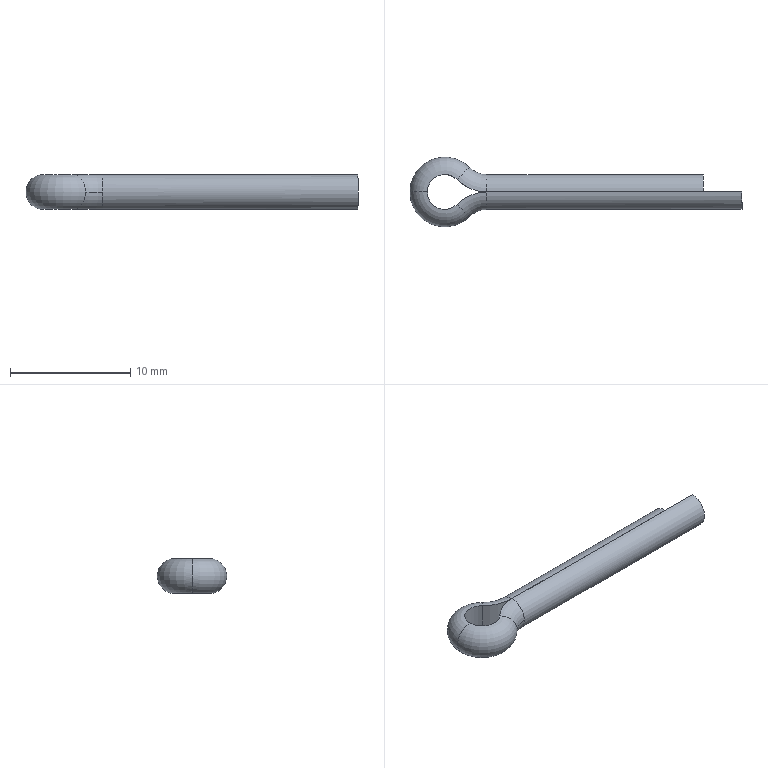Part | SolidWorks | features Sweep 1 | 1 solid | 16 faces | box 27.6 x 5.8 x 2.9 mm | volume 176.57 mm3 | torus 6 | cylinder 6 | plane 4 | commonest cylinder face diameters 2.9 x4 6.998 x2
STEP:
#1=CARTESIAN_POINT('',(6.4,1.45,0.));
#2=VERTEX_POINT('',#1);
#3=CARTESIAN_POINT('',(6.4,0.,1.45));
#4=VERTEX_POINT('',#3);
#5=CARTESIAN_POINT('',(6.4,0.,0.));
#6=DIRECTION('',(1.,0.,0.));
#7=DIRECTION('',(0.,0.,-1.));
#8=AXIS2_PLACEMENT_3D('',#5,#6,#7);
#9=CIRCLE('',#8,1.45);
#10=EDGE_CURVE('',#2,#4,#9,.T.);
#11=ORIENTED_EDGE('',*,*,#10,.F.);
#12=CARTESIAN_POINT('',(4.951,2.05,0.));
#13=VERTEX_POINT('',#12);
#14=CARTESIAN_POINT('',(6.4,3.499,0.));
#15=DIRECTION('',(0.,0.,-1.));
#16=DIRECTION('',(-1.,0.,0.));
#17=AXIS2_PLACEMENT_3D('',#14,#15,#16);
#18=CIRCLE('',#17,2.049);
#19=EDGE_CURVE('',#2,#13,#18,.T.);
#20=ORIENTED_EDGE('',*,*,#19,.T.);
#21=CARTESIAN_POINT('',(3.925,1.025,1.45));
#22=VERTEX_POINT('',#21);
#23=CARTESIAN_POINT('',(3.925,1.025,0.));
#24=DIRECTION('',(0.707,-0.7072,0.));
#25=DIRECTION('',(0.,0.,-1.));
#26=AXIS2_PLACEMENT_3D('',#23,#24,#25);
#27=CIRCLE('',#26,1.45);
#28=EDGE_CURVE('',#13,#22,#27,.T.);
#29=ORIENTED_EDGE('',*,*,#28,.T.);
#30=CARTESIAN_POINT('',(6.4,3.499,1.45));
#31=DIRECTION('',(0.,0.,-1.));
#32=DIRECTION('',(-1.,0.,0.));
#33=AXIS2_PLACEMENT_3D('',#30,#31,#32);
#34=CIRCLE('',#33,3.499);
#35=EDGE_CURVE('',#4,#22,#34,.T.);
#36=ORIENTED_EDGE('',*,*,#35,.F.);
#37=EDGE_LOOP('',(#11,#20,#29,#36));
#38=FACE_OUTER_BOUND('',#37,.T.);
#39=CARTESIAN_POINT('',(6.4,3.499,0.));
#40=DIRECTION('',(0.,0.,-1.));
#41=DIRECTION('',(-1.,0.,0.));
#42=AXIS2_PLACEMENT_3D('',#39,#40,#41);
#43=TOROIDAL_SURFACE('',#42,3.499,1.45);
#44=ADVANCED_FACE('',(#38),#43,.T.);
#45=CARTESIAN_POINT('',(4.951,-2.05,0.));
#46=VERTEX_POINT('',#45);
#47=CARTESIAN_POINT('',(3.925,-1.025,1.45));
#48=VERTEX_POINT('',#47);
#49=CARTESIAN_POINT('',(3.925,-1.025,0.));
#50=DIRECTION('',(-0.707,-0.7072,0.));
#51=DIRECTION('',(0.,0.,-1.));
#52=AXIS2_PLACEMENT_3D('',#49,#50,#51);
#53=CIRCLE('',#52,1.45);
#54=EDGE_CURVE('',#46,#48,#53,.T.);
#55=ORIENTED_EDGE('',*,*,#54,.F.);
#56=CARTESIAN_POINT('',(6.4,-1.45,0.));
#57=VERTEX_POINT('',#56);
#58=CARTESIAN_POINT('',(6.4,-3.499,0.));
#59=DIRECTION('',(0.,0.,-1.));
#60=DIRECTION('',(-1.,0.,0.));
#61=AXIS2_PLACEMENT_3D('',#58,#59,#60);
#62=CIRCLE('',#61,2.049);
#63=EDGE_CURVE('',#46,#57,#62,.T.);
#64=ORIENTED_EDGE('',*,*,#63,.T.);
#65=CARTESIAN_POINT('',(6.4,0.,1.45));
#66=VERTEX_POINT('',#65);
#67=CARTESIAN_POINT('',(6.4,0.,0.));
#68=DIRECTION('',(-1.,0.,0.));
#69=DIRECTION('',(0.,0.,-1.));
#70=AXIS2_PLACEMENT_3D('',#67,#68,#69);
#71=CIRCLE('',#70,1.45);
#72=EDGE_CURVE('',#57,#66,#71,.T.);
#73=ORIENTED_EDGE('',*,*,#72,.T.);
#74=CARTESIAN_POINT('',(6.4,-3.499,1.45));
#75=DIRECTION('',(0.,0.,-1.));
#76=DIRECTION('',(-1.,0.,0.));
#77=AXIS2_PLACEMENT_3D('',#74,#75,#76);
#78=CIRCLE('',#77,3.499);
#79=EDGE_CURVE('',#48,#66,#78,.T.);
#80=ORIENTED_EDGE('',*,*,#79,.F.);
#81=EDGE_LOOP('',(#55,#64,#73,#80));
#82=FACE_OUTER_BOUND('',#81,.T.);
#83=CARTESIAN_POINT('',(6.4,-3.499,0.));
#84=DIRECTION('',(0.,0.,-1.));
#85=DIRECTION('',(-1.,0.,0.));
#86=AXIS2_PLACEMENT_3D('',#83,#84,#85);
#87=TOROIDAL_SURFACE('',#86,3.499,1.45);
#88=ADVANCED_FACE('',(#82),#87,.T.);
#89=CARTESIAN_POINT('',(6.4,0.,-1.45));
#90=VERTEX_POINT('',#89);
#91=CARTESIAN_POINT('',(6.4,0.,0.));
#92=DIRECTION('',(1.,0.,0.));
#93=DIRECTION('',(0.,0.,-1.));
#94=AXIS2_PLACEMENT_3D('',#91,#92,#93);
#95=CIRCLE('',#94,1.45);
#96=EDGE_CURVE('',#90,#2,#95,.T.);
#97=ORIENTED_EDGE('',*,*,#96,.T.);
#98=CARTESIAN_POINT('',(24.4,1.45,0.));
#99=VERTEX_POINT('',#98);
#100=CARTESIAN_POINT('',(6.4,1.45,0.));
#101=DIRECTION('',(1.,0.,0.));
#102=VECTOR('',#101,1000.);
#103=LINE('',#100,#102);
#104=EDGE_CURVE('',#2,#99,#103,.T.);
#105=ORIENTED_EDGE('',*,*,#104,.T.);
#106=CARTESIAN_POINT('',(24.4,0.,-1.45));
#107=VERTEX_POINT('',#106);
#108=CARTESIAN_POINT('',(24.4,0.,0.));
#109=DIRECTION('',(1.,0.,0.));
#110=DIRECTION('',(0.,0.,-1.));
#111=AXIS2_PLACEMENT_3D('',#108,#109,#110);
#112=CIRCLE('',#111,1.45);
#113=EDGE_CURVE('',#107,#99,#112,.T.);
#114=ORIENTED_EDGE('',*,*,#113,.F.);
#115=CARTESIAN_POINT('',(6.4,0.,-1.45));
#116=DIRECTION('',(1.,0.,0.));
#117=VECTOR('',#116,1000.);
#118=LINE('',#115,#117);
#119=EDGE_CURVE('',#90,#107,#118,.T.);
#120=ORIENTED_EDGE('',*,*,#119,.F.);
#121=EDGE_LOOP('',(#97,#105,#114,#120));
#122=FACE_OUTER_BOUND('',#121,.T.);
#123=CARTESIAN_POINT('',(6.4,0.,0.));
#124=DIRECTION('',(1.,0.,0.));
#125=DIRECTION('',(0.,1.,0.));
#126=AXIS2_PLACEMENT_3D('',#123,#124,#125);
#127=CYLINDRICAL_SURFACE('',#126,1.45);
#128=ADVANCED_FACE('',(#122),#127,.T.);
#129=CARTESIAN_POINT('',(3.925,1.025,-1.45));
#130=VERTEX_POINT('',#129);
#131=CARTESIAN_POINT('',(1.45,0.,-1.45));
#132=VERTEX_POINT('',#131);
#133=CARTESIAN_POINT('',(2.9,0.,-1.45));
#134=DIRECTION('',(0.,0.,1.));
#135=DIRECTION('',(1.,0.,0.));
#136=AXIS2_PLACEMENT_3D('',#133,#134,#135);
#137=CIRCLE('',#136,1.45);
#138=EDGE_CURVE('',#130,#132,#137,.T.);
#139=ORIENTED_EDGE('',*,*,#138,.T.);
#140=CARTESIAN_POINT('',(1.45,0.,1.45));
#141=VERTEX_POINT('',#140);
#142=CARTESIAN_POINT('',(1.45,0.,0.));
#143=DIRECTION('',(0.,1.,0.));
#144=DIRECTION('',(-1.,0.,0.));
#145=AXIS2_PLACEMENT_3D('',#142,#143,#144);
#146=CIRCLE('',#145,1.45);
#147=EDGE_CURVE('',#132,#141,#146,.T.);
#148=ORIENTED_EDGE('',*,*,#147,.T.);
#149=CARTESIAN_POINT('',(2.9,0.,1.45));
#150=DIRECTION('',(0.,0.,1.));
#151=DIRECTION('',(1.,0.,0.));
#152=AXIS2_PLACEMENT_3D('',#149,#150,#151);
#153=CIRCLE('',#152,1.45);
#154=EDGE_CURVE('',#22,#141,#153,.T.);
#155=ORIENTED_EDGE('',*,*,#154,.F.);
#156=ORIENTED_EDGE('',*,*,#28,.F.);
#157=CARTESIAN_POINT('',(3.925,1.025,0.));
#158=DIRECTION('',(0.707,-0.7072,0.));
#159=DIRECTION('',(0.,0.,-1.));
#160=AXIS2_PLACEMENT_3D('',#157,#158,#159);
#161=CIRCLE('',#160,1.45);
#162=EDGE_CURVE('',#130,#13,#161,.T.);
#163=ORIENTED_EDGE('',*,*,#162,.F.);
#164=EDGE_LOOP('',(#139,#148,#155,#156,#163));
#165=FACE_OUTER_BOUND('',#164,.T.);
#166=CARTESIAN_POINT('',(2.9,0.,0.));
#167=DIRECTION('',(0.,0.,1.));
#168=DIRECTION('',(1.,0.,0.));
#169=AXIS2_PLACEMENT_3D('',#166,#167,#168);
#170=TOROIDAL_SURFACE('',#169,1.45,1.45);
#171=ADVANCED_FACE('',(#165),#170,.T.);
#172=CARTESIAN_POINT('',(6.4,0.,-1.45));
#173=VERTEX_POINT('',#172);
#174=CARTESIAN_POINT('',(6.4,0.,-1.45));
#175=DIRECTION('',(0.,0.,-1.));
#176=VECTOR('',#175,1000.);
#177=LINE('',#174,#176);
#178=EDGE_CURVE('',#66,#173,#177,.T.);
#179=ORIENTED_EDGE('',*,*,#178,.F.);
#180=CARTESIAN_POINT('',(27.6,0.,1.45));
#181=VERTEX_POINT('',#180);
#182=CARTESIAN_POINT('',(6.4,0.,1.45));
#183=DIRECTION('',(1.,0.,0.));
#184=VECTOR('',#183,1000.);
#185=LINE('',#182,#184);
#186=EDGE_CURVE('',#66,#181,#185,.T.);
#187=ORIENTED_EDGE('',*,*,#186,.T.);
#188=CARTESIAN_POINT('',(27.6,0.,-1.45));
#189=VERTEX_POINT('',#188);
#190=CARTESIAN_POINT('',(27.6,0.,-1.45));
#191=DIRECTION('',(0.,0.,-1.));
#192=VECTOR('',#191,1000.);
#193=LINE('',#190,#192);
#194=EDGE_CURVE('',#181,#189,#193,.T.);
#195=ORIENTED_EDGE('',*,*,#194,.T.);
#196=CARTESIAN_POINT('',(6.4,0.,-1.45));
#197=DIRECTION('',(1.,0.,0.));
#198=VECTOR('',#197,1000.);
#199=LINE('',#196,#198);
#200=EDGE_CURVE('',#173,#189,#199,.T.);
#201=ORIENTED_EDGE('',*,*,#200,.F.);
#202=EDGE_LOOP('',(#179,#187,#195,#201));
#203=FACE_OUTER_BOUND('',#202,.T.);
#204=CARTESIAN_POINT('',(6.4,0.,-1.45));
#205=DIRECTION('',(0.,-1.,0.));
#206=DIRECTION('',(1.,0.,0.));
#207=AXIS2_PLACEMENT_3D('',#204,#205,#206);
#208=PLANE('',#207);
#209=ADVANCED_FACE('',(#203),#208,.F.);
#210=CARTESIAN_POINT('',(6.4,0.,0.));
#211=DIRECTION('',(-1.,0.,0.));
#212=DIRECTION('',(0.,0.,-1.));
#213=AXIS2_PLACEMENT_3D('',#210,#211,#212);
#214=CIRCLE('',#213,1.45);
#215=EDGE_CURVE('',#173,#57,#214,.T.);
#216=ORIENTED_EDGE('',*,*,#215,.F.);
#217=ORIENTED_EDGE('',*,*,#200,.T.);
#218=CARTESIAN_POINT('',(27.6,0.,0.));
#219=DIRECTION('',(-1.,0.,0.));
#220=DIRECTION('',(0.,0.,-1.));
#221=AXIS2_PLACEMENT_3D('',#218,#219,#220);
#222=CIRCLE('',#221,1.45);
#223=EDGE_CURVE('',#189,#181,#222,.T.);
#224=ORIENTED_EDGE('',*,*,#223,.T.);
#225=ORIENTED_EDGE('',*,*,#186,.F.);
#226=ORIENTED_EDGE('',*,*,#72,.F.);
#227=EDGE_LOOP('',(#216,#217,#224,#225,#226));
#228=FACE_OUTER_BOUND('',#227,.T.);
#229=CARTESIAN_POINT('',(6.4,0.,0.));
#230=DIRECTION('',(1.,0.,0.));
#231=DIRECTION('',(0.,1.,0.));
#232=AXIS2_PLACEMENT_3D('',#229,#230,#231);
#233=CYLINDRICAL_SURFACE('',#232,1.45);
#234=ADVANCED_FACE('',(#228),#233,.T.);
#235=CARTESIAN_POINT('',(3.925,-1.025,-1.45));
#236=VERTEX_POINT('',#235);
#237=CARTESIAN_POINT('',(3.925,-1.025,-1.45));
#238=DIRECTION('',(0.,0.,-1.));
#239=VECTOR('',#238,1000.);
#240=LINE('',#237,#239);
#241=EDGE_CURVE('',#48,#236,#240,.T.);
#242=ORIENTED_EDGE('',*,*,#241,.F.);
#243=ORIENTED_EDGE('',*,*,#79,.T.);
#244=ORIENTED_EDGE('',*,*,#178,.T.);
#245=CARTESIAN_POINT('',(6.4,-3.499,-1.45));
#246=DIRECTION('',(0.,0.,-1.));
#247=DIRECTION('',(-1.,0.,0.));
#248=AXIS2_PLACEMENT_3D('',#245,#246,#247);
#249=CIRCLE('',#248,3.499);
#250=EDGE_CURVE('',#236,#173,#249,.T.);
#251=ORIENTED_EDGE('',*,*,#250,.F.);
#252=EDGE_LOOP('',(#242,#243,#244,#251));
#253=FACE_OUTER_BOUND('',#252,.T.);
#254=CARTESIAN_POINT('',(6.4,-3.499,0.));
#255=DIRECTION('',(0.,0.,-1.));
#256=DIRECTION('',(-1.,0.,0.));
#257=AXIS2_PLACEMENT_3D('',#254,#255,#256);
#258=CYLINDRICAL_SURFACE('',#257,3.499);
#259=ADVANCED_FACE('',(#253),#258,.T.);
#260=ORIENTED_EDGE('',*,*,#63,.F.);
#261=CARTESIAN_POINT('',(3.925,-1.025,0.));
#262=DIRECTION('',(-0.707,-0.7072,0.));
#263=DIRECTION('',(0.,0.,-1.));
#264=AXIS2_PLACEMENT_3D('',#261,#262,#263);
#265=CIRCLE('',#264,1.45);
#266=EDGE_CURVE('',#236,#46,#265,.T.);
#267=ORIENTED_EDGE('',*,*,#266,.F.);
#268=ORIENTED_EDGE('',*,*,#250,.T.);
#269=ORIENTED_EDGE('',*,*,#215,.T.);
#270=EDGE_LOOP('',(#260,#267,#268,#269));
#271=FACE_OUTER_BOUND('',#270,.T.);
#272=CARTESIAN_POINT('',(6.4,-3.499,0.));
#273=DIRECTION('',(0.,0.,-1.));
#274=DIRECTION('',(-1.,0.,0.));
#275=AXIS2_PLACEMENT_3D('',#272,#273,#274);
#276=TOROIDAL_SURFACE('',#275,3.499,1.45);
#277=ADVANCED_FACE('',(#271),#276,.T.);
#278=CARTESIAN_POINT('',(3.925,1.025,-1.45));
#279=DIRECTION('',(0.,0.,-1.));
#280=VECTOR('',#279,1000.);
#281=LINE('',#278,#280);
#282=EDGE_CURVE('',#22,#130,#281,.T.);
#283=ORIENTED_EDGE('',*,*,#282,.F.);
#284=ORIENTED_EDGE('',*,*,#154,.T.);
#285=CARTESIAN_POINT('',(2.9,0.,1.45));
#286=DIRECTION('',(0.,0.,1.));
#287=DIRECTION('',(1.,0.,0.));
#288=AXIS2_PLACEMENT_3D('',#285,#286,#287);
#289=CIRCLE('',#288,1.45);
#290=EDGE_CURVE('',#141,#48,#289,.T.);
#291=ORIENTED_EDGE('',*,*,#290,.T.);
#292=ORIENTED_EDGE('',*,*,#241,.T.);
#293=CARTESIAN_POINT('',(2.9,0.,-1.45));
#294=DIRECTION('',(0.,0.,1.));
#295=DIRECTION('',(1.,0.,0.));
#296=AXIS2_PLACEMENT_3D('',#293,#294,#295);
#297=CIRCLE('',#296,1.45);
#298=EDGE_CURVE('',#132,#236,#297,.T.);
#299=ORIENTED_EDGE('',*,*,#298,.F.);
#300=ORIENTED_EDGE('',*,*,#138,.F.);
#301=EDGE_LOOP('',(#283,#284,#291,#292,#299,#300));
#302=FACE_OUTER_BOUND('',#301,.T.);
#303=CARTESIAN_POINT('',(2.9,0.,0.));
#304=DIRECTION('',(0.,0.,1.));
#305=DIRECTION('',(1.,0.,0.));
#306=AXIS2_PLACEMENT_3D('',#303,#304,#305);
#307=CYLINDRICAL_SURFACE('',#306,1.45);
#308=ADVANCED_FACE('',(#302),#307,.F.);
#309=ORIENTED_EDGE('',*,*,#147,.F.);
#310=ORIENTED_EDGE('',*,*,#298,.T.);
#311=ORIENTED_EDGE('',*,*,#266,.T.);
#312=ORIENTED_EDGE('',*,*,#54,.T.);
#313=ORIENTED_EDGE('',*,*,#290,.F.);
#314=EDGE_LOOP('',(#309,#310,#311,#312,#313));
#315=FACE_OUTER_BOUND('',#314,.T.);
#316=CARTESIAN_POINT('',(2.9,0.,0.));
#317=DIRECTION('',(0.,0.,1.));
#318=DIRECTION('',(1.,0.,0.));
#319=AXIS2_PLACEMENT_3D('',#316,#317,#318);
#320=TOROIDAL_SURFACE('',#319,1.45,1.45);
#321=ADVANCED_FACE('',(#315),#320,.T.);
#322=CARTESIAN_POINT('',(6.4,0.,-1.45));
#323=DIRECTION('',(0.,0.,-1.));
#324=VECTOR('',#323,1000.);
#325=LINE('',#322,#324);
#326=EDGE_CURVE('',#4,#90,#325,.T.);
#327=ORIENTED_EDGE('',*,*,#326,.F.);
#328=ORIENTED_EDGE('',*,*,#35,.T.);
#329=ORIENTED_EDGE('',*,*,#282,.T.);
#330=CARTESIAN_POINT('',(6.4,3.499,-1.45));
#331=DIRECTION('',(0.,0.,-1.));
#332=DIRECTION('',(-1.,0.,0.));
#333=AXIS2_PLACEMENT_3D('',#330,#331,#332);
#334=CIRCLE('',#333,3.499);
#335=EDGE_CURVE('',#90,#130,#334,.T.);
#336=ORIENTED_EDGE('',*,*,#335,.F.);
#337=EDGE_LOOP('',(#327,#328,#329,#336));
#338=FACE_OUTER_BOUND('',#337,.T.);
#339=CARTESIAN_POINT('',(6.4,3.499,0.));
#340=DIRECTION('',(0.,0.,-1.));
#341=DIRECTION('',(-1.,0.,0.));
#342=AXIS2_PLACEMENT_3D('',#339,#340,#341);
#343=CYLINDRICAL_SURFACE('',#342,3.499);
#344=ADVANCED_FACE('',(#338),#343,.T.);
#345=ORIENTED_EDGE('',*,*,#19,.F.);
#346=ORIENTED_EDGE('',*,*,#96,.F.);
#347=ORIENTED_EDGE('',*,*,#335,.T.);
#348=ORIENTED_EDGE('',*,*,#162,.T.);
#349=EDGE_LOOP('',(#345,#346,#347,#348));
#350=FACE_OUTER_BOUND('',#349,.T.);
#351=CARTESIAN_POINT('',(6.4,3.499,0.));
#352=DIRECTION('',(0.,0.,-1.));
#353=DIRECTION('',(-1.,0.,0.));
#354=AXIS2_PLACEMENT_3D('',#351,#352,#353);
#355=TOROIDAL_SURFACE('',#354,3.499,1.45);
#356=ADVANCED_FACE('',(#350),#355,.T.);
#357=ORIENTED_EDGE('',*,*,#104,.F.);
#358=ORIENTED_EDGE('',*,*,#10,.T.);
#359=CARTESIAN_POINT('',(24.4,0.,1.45));
#360=VERTEX_POINT('',#359);
#361=CARTESIAN_POINT('',(6.4,0.,1.45));
#362=DIRECTION('',(1.,0.,0.));
#363=VECTOR('',#362,1000.);
#364=LINE('',#361,#363);
#365=EDGE_CURVE('',#4,#360,#364,.T.);
#366=ORIENTED_EDGE('',*,*,#365,.T.);
#367=CARTESIAN_POINT('',(24.4,0.,0.));
#368=DIRECTION('',(1.,0.,0.));
#369=DIRECTION('',(0.,0.,-1.));
#370=AXIS2_PLACEMENT_3D('',#367,#368,#369);
#371=CIRCLE('',#370,1.45);
#372=EDGE_CURVE('',#99,#360,#371,.T.);
#373=ORIENTED_EDGE('',*,*,#372,.F.);
#374=EDGE_LOOP('',(#357,#358,#366,#373));
#375=FACE_OUTER_BOUND('',#374,.T.);
#376=CARTESIAN_POINT('',(6.4,0.,0.));
#377=DIRECTION('',(1.,0.,0.));
#378=DIRECTION('',(0.,1.,0.));
#379=AXIS2_PLACEMENT_3D('',#376,#377,#378);
#380=CYLINDRICAL_SURFACE('',#379,1.45);
#381=ADVANCED_FACE('',(#375),#380,.T.);
#382=CARTESIAN_POINT('',(24.4,0.,-1.45));
#383=DIRECTION('',(0.,0.,-1.));
#384=VECTOR('',#383,1000.);
#385=LINE('',#382,#384);
#386=EDGE_CURVE('',#360,#107,#385,.T.);
#387=ORIENTED_EDGE('',*,*,#386,.F.);
#388=ORIENTED_EDGE('',*,*,#365,.F.);
#389=ORIENTED_EDGE('',*,*,#326,.T.);
#390=ORIENTED_EDGE('',*,*,#119,.T.);
#391=EDGE_LOOP('',(#387,#388,#389,#390));
#392=FACE_OUTER_BOUND('',#391,.T.);
#393=CARTESIAN_POINT('',(6.4,0.,-1.45));
#394=DIRECTION('',(0.,-1.,0.));
#395=DIRECTION('',(1.,0.,0.));
#396=AXIS2_PLACEMENT_3D('',#393,#394,#395);
#397=PLANE('',#396);
#398=ADVANCED_FACE('',(#392),#397,.T.);
#399=ORIENTED_EDGE('',*,*,#223,.F.);
#400=ORIENTED_EDGE('',*,*,#194,.F.);
#401=EDGE_LOOP('',(#399,#400));
#402=FACE_OUTER_BOUND('',#401,.T.);
#403=CARTESIAN_POINT('',(27.6,0.,0.));
#404=DIRECTION('',(-1.,0.,0.));
#405=DIRECTION('',(0.,0.,-1.));
#406=AXIS2_PLACEMENT_3D('',#403,#404,#405);
#407=PLANE('',#406);
#408=ADVANCED_FACE('',(#402),#407,.F.);
#409=ORIENTED_EDGE('',*,*,#113,.T.);
#410=ORIENTED_EDGE('',*,*,#372,.T.);
#411=ORIENTED_EDGE('',*,*,#386,.T.);
#412=EDGE_LOOP('',(#409,#410,#411));
#413=FACE_OUTER_BOUND('',#412,.T.);
#414=CARTESIAN_POINT('',(24.4,0.,0.));
#415=DIRECTION('',(1.,0.,0.));
#416=DIRECTION('',(0.,0.,-1.));
#417=AXIS2_PLACEMENT_3D('',#414,#415,#416);
#418=PLANE('',#417);
#419=ADVANCED_FACE('',(#413),#418,.T.);
#420=CLOSED_SHELL('',(#44,#88,#128,#171,#209,#234,#259,#277,#308,#321,#344,#356,#381,#398,#408,#419));
#421=MANIFOLD_SOLID_BREP('',#420);
#422=CARTESIAN_POINT('',(0.,0.,0.));
#423=DIRECTION('',(0.,0.,1.));
#424=DIRECTION('',(1.,0.,0.));
#425=AXIS2_PLACEMENT_3D('',#422,#423,#424);
#426=(LENGTH_UNIT()NAMED_UNIT(*)SI_UNIT(.MILLI.,.METRE.));
#427=UNCERTAINTY_MEASURE_WITH_UNIT(LENGTH_MEASURE(0.00001),#426,'','');
#428=(NAMED_UNIT(*)PLANE_ANGLE_UNIT()SI_UNIT($,.RADIAN.));
#429=(NAMED_UNIT(*)SI_UNIT($,.STERADIAN.)SOLID_ANGLE_UNIT());
#430=(GEOMETRIC_REPRESENTATION_CONTEXT(3)GLOBAL_UNCERTAINTY_ASSIGNED_CONTEXT((#427))GLOBAL_UNIT_ASSIGNED_CONTEXT((#426,#428,#429))REPRESENTATION_CONTEXT('',''));
#431=ADVANCED_BREP_SHAPE_REPRESENTATION('',(#421,#425),#430);